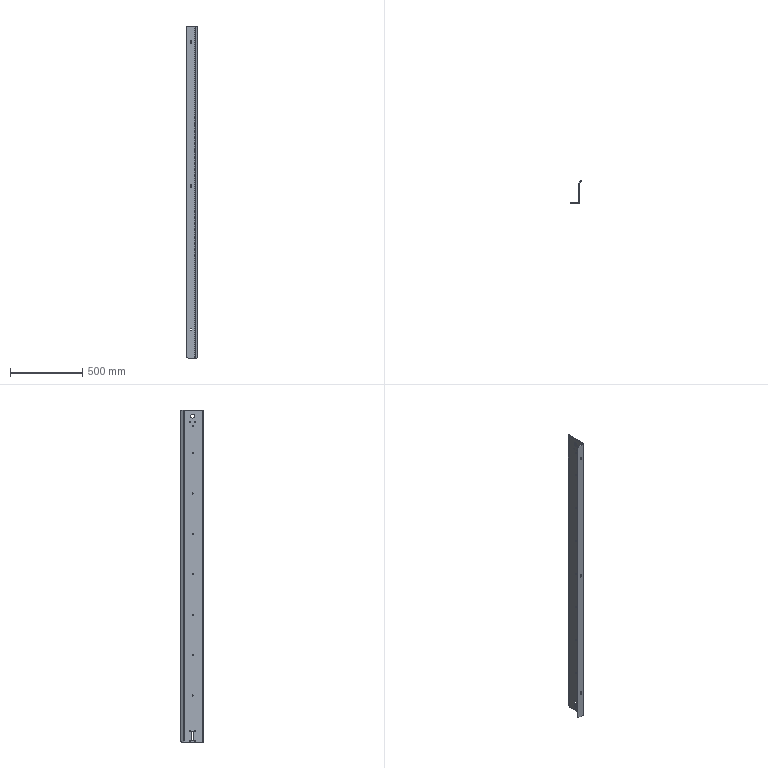Part | SolidWorks | features MirrorStock 1 | 1 solid | 73 faces | box 72.5 x 159.151 x 2300 mm | volume 2459772 mm3 | cylinder 47 | plane 26 | commonest cylinder face diameters 8 x14 5 x8 9 x7 6.8 x6 20 x4 1 x2